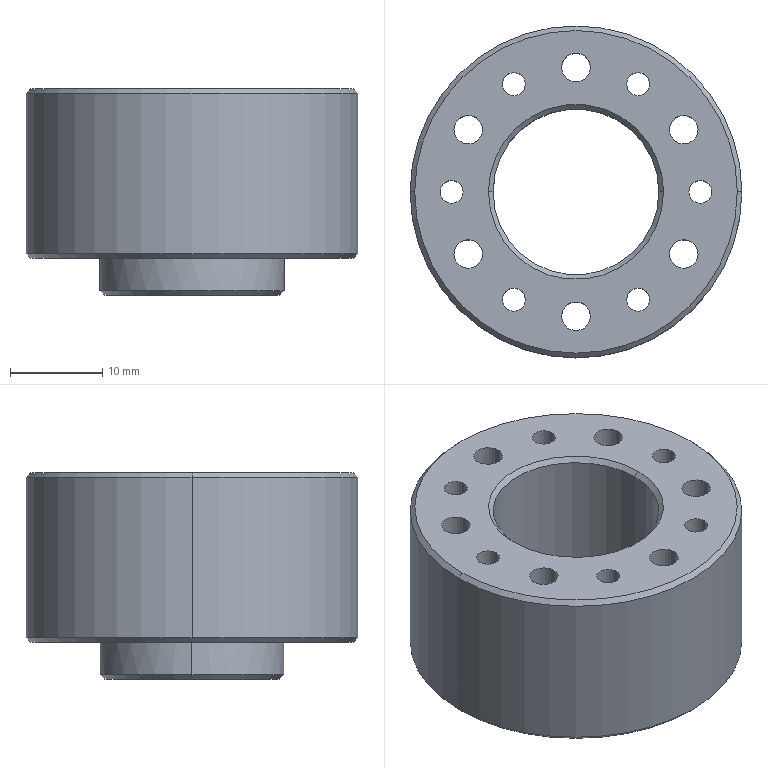Part | SolidWorks | features ICE 2, Chamfer 1, Extrusion 1, HoleWzd 1 | 1 solid | 59 faces | box 36 x 36 x 22.4 mm | volume 11568 mm3 | cylinder 42 | plane 9 | cone 8 | commonest cylinder face diameters 2.5 x12 3.1 x12 7 x12 18 x2 20 x2 36 x2